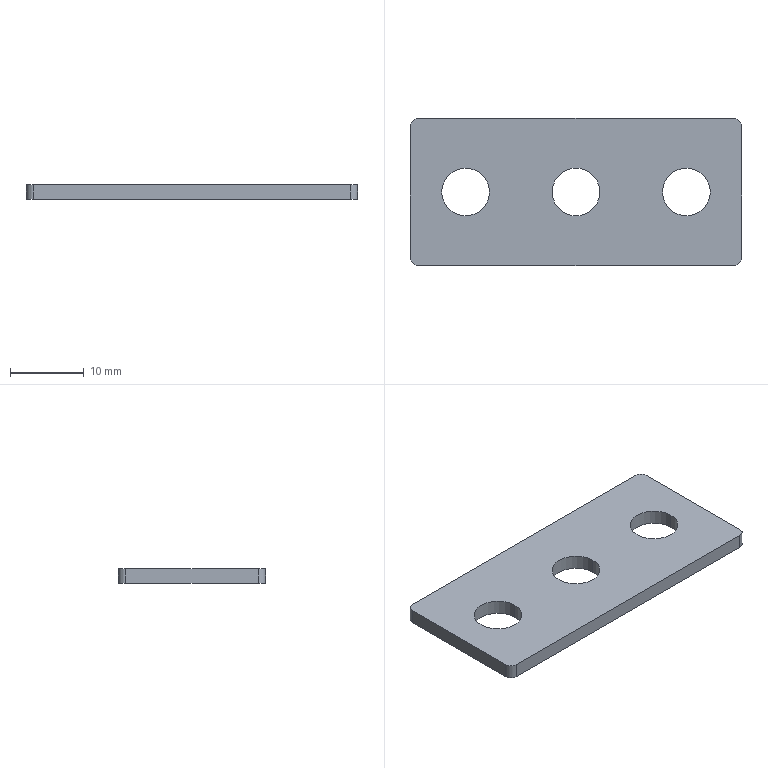Part | STEP file | 601-07-0010 | 1 solid | 16 faces | box 45 x 20 x 2 mm | volume 1599 mm3 | cylinder 10 | plane 6 | commonest cylinder face diameters 6.5 x6 2 x4
STEP:
#1=CARTESIAN_POINT('',(0.,0.,0.));
#2=DIRECTION('',(0.,0.,1.));
#3=DIRECTION('',(1.,0.,0.));
#4=AXIS2_PLACEMENT_3D('',#1,#2,#3);
#5=CARTESIAN_POINT('',(18.25,0.,0.));
#6=VERTEX_POINT('',#5);
#7=CARTESIAN_POINT('',(18.25,0.,2.));
#8=VERTEX_POINT('',#7);
#9=CARTESIAN_POINT('',(18.25,0.,0.));
#10=DIRECTION('',(0.,0.,1.));
#11=VECTOR('',#10,1.);
#12=LINE('',#9,#11);
#13=CARTESIAN_POINT('',(15.,0.,0.));
#14=DIRECTION('',(0.,0.,1.));
#15=DIRECTION('',(1.,0.,0.));
#16=AXIS2_PLACEMENT_3D('',#13,#14,#15);
#17=CYLINDRICAL_SURFACE('',#16,3.25);
#18=CARTESIAN_POINT('',(6.283,0.));
#19=DIRECTION('',(0.,1.));
#20=VECTOR('',#19,1.);
#21=LINE('',#18,#20);
#22=(GEOMETRIC_REPRESENTATION_CONTEXT(2)PARAMETRIC_REPRESENTATION_CONTEXT()REPRESENTATION_CONTEXT('',''));
#23=DEFINITIONAL_REPRESENTATION('',(#21),#22);
#24=PCURVE('',#17,#23);
#25=CARTESIAN_POINT('',(15.,0.,0.));
#26=DIRECTION('',(0.,0.,1.));
#27=DIRECTION('',(1.,0.,0.));
#28=AXIS2_PLACEMENT_3D('',#25,#26,#27);
#29=CYLINDRICAL_SURFACE('',#28,3.25);
#30=CARTESIAN_POINT('',(0.,0.));
#31=DIRECTION('',(0.,1.));
#32=VECTOR('',#31,1.);
#33=LINE('',#30,#32);
#34=(GEOMETRIC_REPRESENTATION_CONTEXT(2)PARAMETRIC_REPRESENTATION_CONTEXT()REPRESENTATION_CONTEXT('',''));
#35=DEFINITIONAL_REPRESENTATION('',(#33),#34);
#36=PCURVE('',#29,#35);
#37=SURFACE_CURVE('',#12,(#24,#36),.PCURVE_S1.);
#38=EDGE_CURVE('',#6,#8,#37,.T.);
#39=ORIENTED_EDGE('',*,*,#38,.T.);
#40=CARTESIAN_POINT('',(11.75,0.,2.));
#41=VERTEX_POINT('',#40);
#42=CARTESIAN_POINT('',(15.,0.,2.));
#43=DIRECTION('',(0.,0.,1.));
#44=DIRECTION('',(1.,0.,0.));
#45=AXIS2_PLACEMENT_3D('',#42,#43,#44);
#46=CIRCLE('',#45,3.25);
#47=CARTESIAN_POINT('',(0.,2.));
#48=DIRECTION('',(1.,0.));
#49=VECTOR('',#48,1.);
#50=LINE('',#47,#49);
#51=(GEOMETRIC_REPRESENTATION_CONTEXT(2)PARAMETRIC_REPRESENTATION_CONTEXT()REPRESENTATION_CONTEXT('',''));
#52=DEFINITIONAL_REPRESENTATION('',(#50),#51);
#53=PCURVE('',#17,#52);
#54=CARTESIAN_POINT('',(22.5,-10.,2.));
#55=DIRECTION('',(0.,0.,1.));
#56=DIRECTION('',(1.,0.,0.));
#57=AXIS2_PLACEMENT_3D('',#54,#55,#56);
#58=PLANE('',#57);
#59=CARTESIAN_POINT('',(-7.5,10.));
#60=DIRECTION('',(1.,0.));
#61=AXIS2_PLACEMENT_2D('',#59,#60);
#62=CIRCLE('',#61,3.25);
#63=(GEOMETRIC_REPRESENTATION_CONTEXT(2)PARAMETRIC_REPRESENTATION_CONTEXT()REPRESENTATION_CONTEXT('',''));
#64=DEFINITIONAL_REPRESENTATION('',(#62),#63);
#65=PCURVE('',#58,#64);
#66=SURFACE_CURVE('',#46,(#53,#65),.PCURVE_S1.);
#67=EDGE_CURVE('',#41,#8,#66,.T.);
#68=ORIENTED_EDGE('',*,*,#67,.F.);
#69=CARTESIAN_POINT('',(11.75,0.,0.));
#70=VERTEX_POINT('',#69);
#71=CARTESIAN_POINT('',(11.75,0.,0.));
#72=DIRECTION('',(0.,0.,1.));
#73=VECTOR('',#72,1.);
#74=LINE('',#71,#73);
#75=CARTESIAN_POINT('',(3.142,0.));
#76=DIRECTION('',(0.,1.));
#77=VECTOR('',#76,1.);
#78=LINE('',#75,#77);
#79=(GEOMETRIC_REPRESENTATION_CONTEXT(2)PARAMETRIC_REPRESENTATION_CONTEXT()REPRESENTATION_CONTEXT('',''));
#80=DEFINITIONAL_REPRESENTATION('',(#78),#79);
#81=PCURVE('',#17,#80);
#82=CARTESIAN_POINT('',(3.142,0.));
#83=DIRECTION('',(0.,1.));
#84=VECTOR('',#83,1.);
#85=LINE('',#82,#84);
#86=(GEOMETRIC_REPRESENTATION_CONTEXT(2)PARAMETRIC_REPRESENTATION_CONTEXT()REPRESENTATION_CONTEXT('',''));
#87=DEFINITIONAL_REPRESENTATION('',(#85),#86);
#88=PCURVE('',#29,#87);
#89=SURFACE_CURVE('',#74,(#81,#88),.PCURVE_S1.);
#90=EDGE_CURVE('',#70,#41,#89,.T.);
#91=ORIENTED_EDGE('',*,*,#90,.F.);
#92=CARTESIAN_POINT('',(15.,0.,0.));
#93=DIRECTION('',(0.,0.,1.));
#94=DIRECTION('',(1.,0.,0.));
#95=AXIS2_PLACEMENT_3D('',#92,#93,#94);
#96=CIRCLE('',#95,3.25);
#97=CARTESIAN_POINT('',(0.,0.));
#98=DIRECTION('',(1.,0.));
#99=VECTOR('',#98,1.);
#100=LINE('',#97,#99);
#101=(GEOMETRIC_REPRESENTATION_CONTEXT(2)PARAMETRIC_REPRESENTATION_CONTEXT()REPRESENTATION_CONTEXT('',''));
#102=DEFINITIONAL_REPRESENTATION('',(#100),#101);
#103=PCURVE('',#17,#102);
#104=CARTESIAN_POINT('',(22.5,-10.,0.));
#105=DIRECTION('',(0.,0.,1.));
#106=DIRECTION('',(1.,0.,0.));
#107=AXIS2_PLACEMENT_3D('',#104,#105,#106);
#108=PLANE('',#107);
#109=CARTESIAN_POINT('',(-7.5,10.));
#110=DIRECTION('',(1.,0.));
#111=AXIS2_PLACEMENT_2D('',#109,#110);
#112=CIRCLE('',#111,3.25);
#113=(GEOMETRIC_REPRESENTATION_CONTEXT(2)PARAMETRIC_REPRESENTATION_CONTEXT()REPRESENTATION_CONTEXT('',''));
#114=DEFINITIONAL_REPRESENTATION('',(#112),#113);
#115=PCURVE('',#108,#114);
#116=SURFACE_CURVE('',#96,(#103,#115),.PCURVE_S1.);
#117=EDGE_CURVE('',#70,#6,#116,.T.);
#118=ORIENTED_EDGE('',*,*,#117,.T.);
#119=EDGE_LOOP('',(#39,#68,#91,#118));
#120=FACE_BOUND('',#119,.F.);
#121=ADVANCED_FACE('',(#120),#17,.F.);
#122=CARTESIAN_POINT('',(3.25,0.,0.));
#123=VERTEX_POINT('',#122);
#124=CARTESIAN_POINT('',(3.25,0.,2.));
#125=VERTEX_POINT('',#124);
#126=CARTESIAN_POINT('',(3.25,0.,0.));
#127=DIRECTION('',(0.,0.,1.));
#128=VECTOR('',#127,1.);
#129=LINE('',#126,#128);
#130=CARTESIAN_POINT('',(0.,0.,0.));
#131=DIRECTION('',(0.,0.,1.));
#132=DIRECTION('',(1.,0.,0.));
#133=AXIS2_PLACEMENT_3D('',#130,#131,#132);
#134=CYLINDRICAL_SURFACE('',#133,3.25);
#135=CARTESIAN_POINT('',(6.283,0.));
#136=DIRECTION('',(0.,1.));
#137=VECTOR('',#136,1.);
#138=LINE('',#135,#137);
#139=(GEOMETRIC_REPRESENTATION_CONTEXT(2)PARAMETRIC_REPRESENTATION_CONTEXT()REPRESENTATION_CONTEXT('',''));
#140=DEFINITIONAL_REPRESENTATION('',(#138),#139);
#141=PCURVE('',#134,#140);
#142=CARTESIAN_POINT('',(0.,0.,0.));
#143=DIRECTION('',(0.,0.,1.));
#144=DIRECTION('',(1.,0.,0.));
#145=AXIS2_PLACEMENT_3D('',#142,#143,#144);
#146=CYLINDRICAL_SURFACE('',#145,3.25);
#147=CARTESIAN_POINT('',(0.,0.));
#148=DIRECTION('',(0.,1.));
#149=VECTOR('',#148,1.);
#150=LINE('',#147,#149);
#151=(GEOMETRIC_REPRESENTATION_CONTEXT(2)PARAMETRIC_REPRESENTATION_CONTEXT()REPRESENTATION_CONTEXT('',''));
#152=DEFINITIONAL_REPRESENTATION('',(#150),#151);
#153=PCURVE('',#146,#152);
#154=SURFACE_CURVE('',#129,(#141,#153),.PCURVE_S1.);
#155=EDGE_CURVE('',#123,#125,#154,.T.);
#156=ORIENTED_EDGE('',*,*,#155,.T.);
#157=CARTESIAN_POINT('',(-3.25,0.,2.));
#158=VERTEX_POINT('',#157);
#159=CARTESIAN_POINT('',(0.,0.,2.));
#160=DIRECTION('',(0.,0.,1.));
#161=DIRECTION('',(1.,0.,0.));
#162=AXIS2_PLACEMENT_3D('',#159,#160,#161);
#163=CIRCLE('',#162,3.25);
#164=CARTESIAN_POINT('',(0.,2.));
#165=DIRECTION('',(1.,0.));
#166=VECTOR('',#165,1.);
#167=LINE('',#164,#166);
#168=(GEOMETRIC_REPRESENTATION_CONTEXT(2)PARAMETRIC_REPRESENTATION_CONTEXT()REPRESENTATION_CONTEXT('',''));
#169=DEFINITIONAL_REPRESENTATION('',(#167),#168);
#170=PCURVE('',#134,#169);
#171=CARTESIAN_POINT('',(-22.5,10.));
#172=DIRECTION('',(1.,0.));
#173=AXIS2_PLACEMENT_2D('',#171,#172);
#174=CIRCLE('',#173,3.25);
#175=(GEOMETRIC_REPRESENTATION_CONTEXT(2)PARAMETRIC_REPRESENTATION_CONTEXT()REPRESENTATION_CONTEXT('',''));
#176=DEFINITIONAL_REPRESENTATION('',(#174),#175);
#177=PCURVE('',#58,#176);
#178=SURFACE_CURVE('',#163,(#170,#177),.PCURVE_S1.);
#179=EDGE_CURVE('',#158,#125,#178,.T.);
#180=ORIENTED_EDGE('',*,*,#179,.F.);
#181=CARTESIAN_POINT('',(-3.25,0.,0.));
#182=VERTEX_POINT('',#181);
#183=CARTESIAN_POINT('',(-3.25,0.,0.));
#184=DIRECTION('',(0.,0.,1.));
#185=VECTOR('',#184,1.);
#186=LINE('',#183,#185);
#187=CARTESIAN_POINT('',(3.142,0.));
#188=DIRECTION('',(0.,1.));
#189=VECTOR('',#188,1.);
#190=LINE('',#187,#189);
#191=(GEOMETRIC_REPRESENTATION_CONTEXT(2)PARAMETRIC_REPRESENTATION_CONTEXT()REPRESENTATION_CONTEXT('',''));
#192=DEFINITIONAL_REPRESENTATION('',(#190),#191);
#193=PCURVE('',#134,#192);
#194=CARTESIAN_POINT('',(3.142,0.));
#195=DIRECTION('',(0.,1.));
#196=VECTOR('',#195,1.);
#197=LINE('',#194,#196);
#198=(GEOMETRIC_REPRESENTATION_CONTEXT(2)PARAMETRIC_REPRESENTATION_CONTEXT()REPRESENTATION_CONTEXT('',''));
#199=DEFINITIONAL_REPRESENTATION('',(#197),#198);
#200=PCURVE('',#146,#199);
#201=SURFACE_CURVE('',#186,(#193,#200),.PCURVE_S1.);
#202=EDGE_CURVE('',#182,#158,#201,.T.);
#203=ORIENTED_EDGE('',*,*,#202,.F.);
#204=CARTESIAN_POINT('',(0.,0.,0.));
#205=DIRECTION('',(0.,0.,1.));
#206=DIRECTION('',(1.,0.,0.));
#207=AXIS2_PLACEMENT_3D('',#204,#205,#206);
#208=CIRCLE('',#207,3.25);
#209=CARTESIAN_POINT('',(0.,0.));
#210=DIRECTION('',(1.,0.));
#211=VECTOR('',#210,1.);
#212=LINE('',#209,#211);
#213=(GEOMETRIC_REPRESENTATION_CONTEXT(2)PARAMETRIC_REPRESENTATION_CONTEXT()REPRESENTATION_CONTEXT('',''));
#214=DEFINITIONAL_REPRESENTATION('',(#212),#213);
#215=PCURVE('',#134,#214);
#216=CARTESIAN_POINT('',(-22.5,10.));
#217=DIRECTION('',(1.,0.));
#218=AXIS2_PLACEMENT_2D('',#216,#217);
#219=CIRCLE('',#218,3.25);
#220=(GEOMETRIC_REPRESENTATION_CONTEXT(2)PARAMETRIC_REPRESENTATION_CONTEXT()REPRESENTATION_CONTEXT('',''));
#221=DEFINITIONAL_REPRESENTATION('',(#219),#220);
#222=PCURVE('',#108,#221);
#223=SURFACE_CURVE('',#208,(#215,#222),.PCURVE_S1.);
#224=EDGE_CURVE('',#182,#123,#223,.T.);
#225=ORIENTED_EDGE('',*,*,#224,.T.);
#226=EDGE_LOOP('',(#156,#180,#203,#225));
#227=FACE_BOUND('',#226,.F.);
#228=ADVANCED_FACE('',(#227),#134,.F.);
#229=CARTESIAN_POINT('',(-11.75,0.,0.));
#230=VERTEX_POINT('',#229);
#231=CARTESIAN_POINT('',(-11.75,0.,2.));
#232=VERTEX_POINT('',#231);
#233=CARTESIAN_POINT('',(-11.75,0.,0.));
#234=DIRECTION('',(0.,0.,1.));
#235=VECTOR('',#234,1.);
#236=LINE('',#233,#235);
#237=CARTESIAN_POINT('',(-15.,0.,0.));
#238=DIRECTION('',(0.,0.,1.));
#239=DIRECTION('',(1.,0.,0.));
#240=AXIS2_PLACEMENT_3D('',#237,#238,#239);
#241=CYLINDRICAL_SURFACE('',#240,3.25);
#242=CARTESIAN_POINT('',(6.283,0.));
#243=DIRECTION('',(0.,1.));
#244=VECTOR('',#243,1.);
#245=LINE('',#242,#244);
#246=(GEOMETRIC_REPRESENTATION_CONTEXT(2)PARAMETRIC_REPRESENTATION_CONTEXT()REPRESENTATION_CONTEXT('',''));
#247=DEFINITIONAL_REPRESENTATION('',(#245),#246);
#248=PCURVE('',#241,#247);
#249=CARTESIAN_POINT('',(-15.,0.,0.));
#250=DIRECTION('',(0.,0.,1.));
#251=DIRECTION('',(1.,0.,0.));
#252=AXIS2_PLACEMENT_3D('',#249,#250,#251);
#253=CYLINDRICAL_SURFACE('',#252,3.25);
#254=CARTESIAN_POINT('',(0.,0.));
#255=DIRECTION('',(0.,1.));
#256=VECTOR('',#255,1.);
#257=LINE('',#254,#256);
#258=(GEOMETRIC_REPRESENTATION_CONTEXT(2)PARAMETRIC_REPRESENTATION_CONTEXT()REPRESENTATION_CONTEXT('',''));
#259=DEFINITIONAL_REPRESENTATION('',(#257),#258);
#260=PCURVE('',#253,#259);
#261=SURFACE_CURVE('',#236,(#248,#260),.PCURVE_S1.);
#262=EDGE_CURVE('',#230,#232,#261,.T.);
#263=ORIENTED_EDGE('',*,*,#262,.T.);
#264=CARTESIAN_POINT('',(-18.25,0.,2.));
#265=VERTEX_POINT('',#264);
#266=CARTESIAN_POINT('',(-15.,0.,2.));
#267=DIRECTION('',(0.,0.,1.));
#268=DIRECTION('',(1.,0.,0.));
#269=AXIS2_PLACEMENT_3D('',#266,#267,#268);
#270=CIRCLE('',#269,3.25);
#271=CARTESIAN_POINT('',(0.,2.));
#272=DIRECTION('',(1.,0.));
#273=VECTOR('',#272,1.);
#274=LINE('',#271,#273);
#275=(GEOMETRIC_REPRESENTATION_CONTEXT(2)PARAMETRIC_REPRESENTATION_CONTEXT()REPRESENTATION_CONTEXT('',''));
#276=DEFINITIONAL_REPRESENTATION('',(#274),#275);
#277=PCURVE('',#241,#276);
#278=CARTESIAN_POINT('',(-37.5,10.));
#279=DIRECTION('',(1.,0.));
#280=AXIS2_PLACEMENT_2D('',#278,#279);
#281=CIRCLE('',#280,3.25);
#282=(GEOMETRIC_REPRESENTATION_CONTEXT(2)PARAMETRIC_REPRESENTATION_CONTEXT()REPRESENTATION_CONTEXT('',''));
#283=DEFINITIONAL_REPRESENTATION('',(#281),#282);
#284=PCURVE('',#58,#283);
#285=SURFACE_CURVE('',#270,(#277,#284),.PCURVE_S1.);
#286=EDGE_CURVE('',#265,#232,#285,.T.);
#287=ORIENTED_EDGE('',*,*,#286,.F.);
#288=CARTESIAN_POINT('',(-18.25,0.,0.));
#289=VERTEX_POINT('',#288);
#290=CARTESIAN_POINT('',(-18.25,0.,0.));
#291=DIRECTION('',(0.,0.,1.));
#292=VECTOR('',#291,1.);
#293=LINE('',#290,#292);
#294=CARTESIAN_POINT('',(3.142,0.));
#295=DIRECTION('',(0.,1.));
#296=VECTOR('',#295,1.);
#297=LINE('',#294,#296);
#298=(GEOMETRIC_REPRESENTATION_CONTEXT(2)PARAMETRIC_REPRESENTATION_CONTEXT()REPRESENTATION_CONTEXT('',''));
#299=DEFINITIONAL_REPRESENTATION('',(#297),#298);
#300=PCURVE('',#241,#299);
#301=CARTESIAN_POINT('',(3.142,0.));
#302=DIRECTION('',(0.,1.));
#303=VECTOR('',#302,1.);
#304=LINE('',#301,#303);
#305=(GEOMETRIC_REPRESENTATION_CONTEXT(2)PARAMETRIC_REPRESENTATION_CONTEXT()REPRESENTATION_CONTEXT('',''));
#306=DEFINITIONAL_REPRESENTATION('',(#304),#305);
#307=PCURVE('',#253,#306);
#308=SURFACE_CURVE('',#293,(#300,#307),.PCURVE_S1.);
#309=EDGE_CURVE('',#289,#265,#308,.T.);
#310=ORIENTED_EDGE('',*,*,#309,.F.);
#311=CARTESIAN_POINT('',(-15.,0.,0.));
#312=DIRECTION('',(0.,0.,1.));
#313=DIRECTION('',(1.,0.,0.));
#314=AXIS2_PLACEMENT_3D('',#311,#312,#313);
#315=CIRCLE('',#314,3.25);
#316=CARTESIAN_POINT('',(0.,0.));
#317=DIRECTION('',(1.,0.));
#318=VECTOR('',#317,1.);
#319=LINE('',#316,#318);
#320=(GEOMETRIC_REPRESENTATION_CONTEXT(2)PARAMETRIC_REPRESENTATION_CONTEXT()REPRESENTATION_CONTEXT('',''));
#321=DEFINITIONAL_REPRESENTATION('',(#319),#320);
#322=PCURVE('',#241,#321);
#323=CARTESIAN_POINT('',(-37.5,10.));
#324=DIRECTION('',(1.,0.));
#325=AXIS2_PLACEMENT_2D('',#323,#324);
#326=CIRCLE('',#325,3.25);
#327=(GEOMETRIC_REPRESENTATION_CONTEXT(2)PARAMETRIC_REPRESENTATION_CONTEXT()REPRESENTATION_CONTEXT('',''));
#328=DEFINITIONAL_REPRESENTATION('',(#326),#327);
#329=PCURVE('',#108,#328);
#330=SURFACE_CURVE('',#315,(#322,#329),.PCURVE_S1.);
#331=EDGE_CURVE('',#289,#230,#330,.T.);
#332=ORIENTED_EDGE('',*,*,#331,.T.);
#333=EDGE_LOOP('',(#263,#287,#310,#332));
#334=FACE_BOUND('',#333,.F.);
#335=ADVANCED_FACE('',(#334),#241,.F.);
#336=CARTESIAN_POINT('',(22.5,-9.,0.));
#337=VERTEX_POINT('',#336);
#338=CARTESIAN_POINT('',(22.5,9.,0.));
#339=VERTEX_POINT('',#338);
#340=CARTESIAN_POINT('',(22.5,10.,0.));
#341=DIRECTION('',(0.,1.,0.));
#342=VECTOR('',#341,1.);
#343=LINE('',#340,#342);
#344=CARTESIAN_POINT('',(22.5,10.,2.));
#345=DIRECTION('',(-1.,0.,0.));
#346=DIRECTION('',(0.,-1.,0.));
#347=AXIS2_PLACEMENT_3D('',#344,#345,#346);
#348=PLANE('',#347);
#349=CARTESIAN_POINT('',(0.,-2.));
#350=DIRECTION('',(-1.,0.));
#351=VECTOR('',#350,1.);
#352=LINE('',#349,#351);
#353=(GEOMETRIC_REPRESENTATION_CONTEXT(2)PARAMETRIC_REPRESENTATION_CONTEXT()REPRESENTATION_CONTEXT('',''));
#354=DEFINITIONAL_REPRESENTATION('',(#352),#353);
#355=PCURVE('',#348,#354);
#356=CARTESIAN_POINT('',(0.,20.));
#357=DIRECTION('',(0.,1.));
#358=VECTOR('',#357,1.);
#359=LINE('',#356,#358);
#360=(GEOMETRIC_REPRESENTATION_CONTEXT(2)PARAMETRIC_REPRESENTATION_CONTEXT()REPRESENTATION_CONTEXT('',''));
#361=DEFINITIONAL_REPRESENTATION('',(#359),#360);
#362=PCURVE('',#108,#361);
#363=SURFACE_CURVE('',#343,(#355,#362),.PCURVE_S1.);
#364=EDGE_CURVE('',#337,#339,#363,.T.);
#365=ORIENTED_EDGE('',*,*,#364,.T.);
#366=CARTESIAN_POINT('',(22.5,9.,2.));
#367=VERTEX_POINT('',#366);
#368=CARTESIAN_POINT('',(22.5,9.,2.));
#369=DIRECTION('',(0.,0.,1.));
#370=VECTOR('',#369,1.);
#371=LINE('',#368,#370);
#372=CARTESIAN_POINT('',(1.,0.));
#373=DIRECTION('',(0.,1.));
#374=VECTOR('',#373,1.);
#375=LINE('',#372,#374);
#376=(GEOMETRIC_REPRESENTATION_CONTEXT(2)PARAMETRIC_REPRESENTATION_CONTEXT()REPRESENTATION_CONTEXT('',''));
#377=DEFINITIONAL_REPRESENTATION('',(#375),#376);
#378=PCURVE('',#348,#377);
#379=CARTESIAN_POINT('',(21.5,9.,2.));
#380=DIRECTION('',(0.,0.,-1.));
#381=DIRECTION('',(-1.,0.,0.));
#382=AXIS2_PLACEMENT_3D('',#379,#380,#381);
#383=CYLINDRICAL_SURFACE('',#382,1.);
#384=CARTESIAN_POINT('',(3.142,0.));
#385=DIRECTION('',(0.,-1.));
#386=VECTOR('',#385,1.);
#387=LINE('',#384,#386);
#388=(GEOMETRIC_REPRESENTATION_CONTEXT(2)PARAMETRIC_REPRESENTATION_CONTEXT()REPRESENTATION_CONTEXT('',''));
#389=DEFINITIONAL_REPRESENTATION('',(#387),#388);
#390=PCURVE('',#383,#389);
#391=SURFACE_CURVE('',#371,(#378,#390),.PCURVE_S1.);
#392=EDGE_CURVE('',#339,#367,#391,.T.);
#393=ORIENTED_EDGE('',*,*,#392,.T.);
#394=CARTESIAN_POINT('',(22.5,-9.,2.));
#395=VERTEX_POINT('',#394);
#396=CARTESIAN_POINT('',(22.5,10.,2.));
#397=DIRECTION('',(0.,1.,0.));
#398=VECTOR('',#397,1.);
#399=LINE('',#396,#398);
#400=CARTESIAN_POINT('',(0.,0.));
#401=DIRECTION('',(-1.,0.));
#402=VECTOR('',#401,1.);
#403=LINE('',#400,#402);
#404=(GEOMETRIC_REPRESENTATION_CONTEXT(2)PARAMETRIC_REPRESENTATION_CONTEXT()REPRESENTATION_CONTEXT('',''));
#405=DEFINITIONAL_REPRESENTATION('',(#403),#404);
#406=PCURVE('',#348,#405);
#407=CARTESIAN_POINT('',(0.,20.));
#408=DIRECTION('',(0.,1.));
#409=VECTOR('',#408,1.);
#410=LINE('',#407,#409);
#411=(GEOMETRIC_REPRESENTATION_CONTEXT(2)PARAMETRIC_REPRESENTATION_CONTEXT()REPRESENTATION_CONTEXT('',''));
#412=DEFINITIONAL_REPRESENTATION('',(#410),#411);
#413=PCURVE('',#58,#412);
#414=SURFACE_CURVE('',#399,(#406,#413),.PCURVE_S1.);
#415=EDGE_CURVE('',#395,#367,#414,.T.);
#416=ORIENTED_EDGE('',*,*,#415,.F.);
#417=CARTESIAN_POINT('',(22.5,-9.,2.));
#418=DIRECTION('',(0.,0.,-1.));
#419=VECTOR('',#418,1.);
#420=LINE('',#417,#419);
#421=CARTESIAN_POINT('',(19.,0.));
#422=DIRECTION('',(0.,-1.));
#423=VECTOR('',#422,1.);
#424=LINE('',#421,#423);
#425=(GEOMETRIC_REPRESENTATION_CONTEXT(2)PARAMETRIC_REPRESENTATION_CONTEXT()REPRESENTATION_CONTEXT('',''));
#426=DEFINITIONAL_REPRESENTATION('',(#424),#425);
#427=PCURVE('',#348,#426);
#428=CARTESIAN_POINT('',(21.5,-9.,2.));
#429=DIRECTION('',(0.,0.,-1.));
#430=DIRECTION('',(-1.,0.,0.));
#431=AXIS2_PLACEMENT_3D('',#428,#429,#430);
#432=CYLINDRICAL_SURFACE('',#431,1.);
#433=CARTESIAN_POINT('',(3.142,0.));
#434=DIRECTION('',(0.,1.));
#435=VECTOR('',#434,1.);
#436=LINE('',#433,#435);
#437=(GEOMETRIC_REPRESENTATION_CONTEXT(2)PARAMETRIC_REPRESENTATION_CONTEXT()REPRESENTATION_CONTEXT('',''));
#438=DEFINITIONAL_REPRESENTATION('',(#436),#437);
#439=PCURVE('',#432,#438);
#440=SURFACE_CURVE('',#420,(#427,#439),.PCURVE_S1.);
#441=EDGE_CURVE('',#395,#337,#440,.T.);
#442=ORIENTED_EDGE('',*,*,#441,.T.);
#443=EDGE_LOOP('',(#365,#393,#416,#442));
#444=FACE_BOUND('',#443,.T.);
#445=ADVANCED_FACE('',(#444),#348,.F.);
#446=CARTESIAN_POINT('',(21.5,10.,0.));
#447=VERTEX_POINT('',#446);
#448=CARTESIAN_POINT('',(-21.5,10.,0.));
#449=VERTEX_POINT('',#448);
#450=CARTESIAN_POINT('',(-22.5,10.,0.));
#451=DIRECTION('',(-1.,0.,0.));
#452=VECTOR('',#451,1.);
#453=LINE('',#450,#452);
#454=CARTESIAN_POINT('',(-22.5,10.,2.));
#455=DIRECTION('',(0.,-1.,0.));
#456=DIRECTION('',(0.,0.,-1.));
#457=AXIS2_PLACEMENT_3D('',#454,#455,#456);
#458=PLANE('',#457);
#459=CARTESIAN_POINT('',(2.,0.));
#460=DIRECTION('',(0.,-1.));
#461=VECTOR('',#460,1.);
#462=LINE('',#459,#461);
#463=(GEOMETRIC_REPRESENTATION_CONTEXT(2)PARAMETRIC_REPRESENTATION_CONTEXT()REPRESENTATION_CONTEXT('',''));
#464=DEFINITIONAL_REPRESENTATION('',(#462),#463);
#465=PCURVE('',#458,#464);
#466=CARTESIAN_POINT('',(-45.,20.));
#467=DIRECTION('',(-1.,0.));
#468=VECTOR('',#467,1.);
#469=LINE('',#466,#468);
#470=(GEOMETRIC_REPRESENTATION_CONTEXT(2)PARAMETRIC_REPRESENTATION_CONTEXT()REPRESENTATION_CONTEXT('',''));
#471=DEFINITIONAL_REPRESENTATION('',(#469),#470);
#472=PCURVE('',#108,#471);
#473=SURFACE_CURVE('',#453,(#465,#472),.PCURVE_S1.);
#474=EDGE_CURVE('',#447,#449,#473,.T.);
#475=ORIENTED_EDGE('',*,*,#474,.T.);
#476=CARTESIAN_POINT('',(-21.5,10.,2.));
#477=VERTEX_POINT('',#476);
#478=CARTESIAN_POINT('',(-21.5,10.,2.));
#479=DIRECTION('',(0.,0.,1.));
#480=VECTOR('',#479,1.);
#481=LINE('',#478,#480);
#482=CARTESIAN_POINT('',(0.,1.));
#483=DIRECTION('',(-1.,0.));
#484=VECTOR('',#483,1.);
#485=LINE('',#482,#484);
#486=(GEOMETRIC_REPRESENTATION_CONTEXT(2)PARAMETRIC_REPRESENTATION_CONTEXT()REPRESENTATION_CONTEXT('',''));
#487=DEFINITIONAL_REPRESENTATION('',(#485),#486);
#488=PCURVE('',#458,#487);
#489=CARTESIAN_POINT('',(-21.5,9.,2.));
#490=DIRECTION('',(0.,0.,-1.));
#491=DIRECTION('',(-1.,0.,0.));
#492=AXIS2_PLACEMENT_3D('',#489,#490,#491);
#493=CYLINDRICAL_SURFACE('',#492,1.);
#494=CARTESIAN_POINT('',(1.571,0.));
#495=DIRECTION('',(0.,-1.));
#496=VECTOR('',#495,1.);
#497=LINE('',#494,#496);
#498=(GEOMETRIC_REPRESENTATION_CONTEXT(2)PARAMETRIC_REPRESENTATION_CONTEXT()REPRESENTATION_CONTEXT('',''));
#499=DEFINITIONAL_REPRESENTATION('',(#497),#498);
#500=PCURVE('',#493,#499);
#501=SURFACE_CURVE('',#481,(#488,#500),.PCURVE_S1.);
#502=EDGE_CURVE('',#449,#477,#501,.T.);
#503=ORIENTED_EDGE('',*,*,#502,.T.);
#504=CARTESIAN_POINT('',(21.5,10.,2.));
#505=VERTEX_POINT('',#504);
#506=CARTESIAN_POINT('',(-22.5,10.,2.));
#507=DIRECTION('',(-1.,0.,0.));
#508=VECTOR('',#507,1.);
#509=LINE('',#506,#508);
#510=CARTESIAN_POINT('',(0.,0.));
#511=DIRECTION('',(0.,-1.));
#512=VECTOR('',#511,1.);
#513=LINE('',#510,#512);
#514=(GEOMETRIC_REPRESENTATION_CONTEXT(2)PARAMETRIC_REPRESENTATION_CONTEXT()REPRESENTATION_CONTEXT('',''));
#515=DEFINITIONAL_REPRESENTATION('',(#513),#514);
#516=PCURVE('',#458,#515);
#517=CARTESIAN_POINT('',(-45.,20.));
#518=DIRECTION('',(-1.,0.));
#519=VECTOR('',#518,1.);
#520=LINE('',#517,#519);
#521=(GEOMETRIC_REPRESENTATION_CONTEXT(2)PARAMETRIC_REPRESENTATION_CONTEXT()REPRESENTATION_CONTEXT('',''));
#522=DEFINITIONAL_REPRESENTATION('',(#520),#521);
#523=PCURVE('',#58,#522);
#524=SURFACE_CURVE('',#509,(#516,#523),.PCURVE_S1.);
#525=EDGE_CURVE('',#505,#477,#524,.T.);
#526=ORIENTED_EDGE('',*,*,#525,.F.);
#527=CARTESIAN_POINT('',(21.5,10.,2.));
#528=DIRECTION('',(0.,0.,-1.));
#529=VECTOR('',#528,1.);
#530=LINE('',#527,#529);
#531=CARTESIAN_POINT('',(0.,44.));
#532=DIRECTION('',(1.,0.));
#533=VECTOR('',#532,1.);
#534=LINE('',#531,#533);
#535=(GEOMETRIC_REPRESENTATION_CONTEXT(2)PARAMETRIC_REPRESENTATION_CONTEXT()REPRESENTATION_CONTEXT('',''));
#536=DEFINITIONAL_REPRESENTATION('',(#534),#535);
#537=PCURVE('',#458,#536);
#538=CARTESIAN_POINT('',(1.571,0.));
#539=DIRECTION('',(0.,1.));
#540=VECTOR('',#539,1.);
#541=LINE('',#538,#540);
#542=(GEOMETRIC_REPRESENTATION_CONTEXT(2)PARAMETRIC_REPRESENTATION_CONTEXT()REPRESENTATION_CONTEXT('',''));
#543=DEFINITIONAL_REPRESENTATION('',(#541),#542);
#544=PCURVE('',#383,#543);
#545=SURFACE_CURVE('',#530,(#537,#544),.PCURVE_S1.);
#546=EDGE_CURVE('',#505,#447,#545,.T.);
#547=ORIENTED_EDGE('',*,*,#546,.T.);
#548=EDGE_LOOP('',(#475,#503,#526,#547));
#549=FACE_BOUND('',#548,.T.);
#550=ADVANCED_FACE('',(#549),#458,.F.);
#551=CARTESIAN_POINT('',(-22.5,9.,0.));
#552=VERTEX_POINT('',#551);
#553=CARTESIAN_POINT('',(-22.5,-9.,0.));
#554=VERTEX_POINT('',#553);
#555=CARTESIAN_POINT('',(-22.5,10.,0.));
#556=DIRECTION('',(0.,-1.,0.));
#557=VECTOR('',#556,1.);
#558=LINE('',#555,#557);
#559=CARTESIAN_POINT('',(-22.5,10.,2.));
#560=DIRECTION('',(1.,0.,0.));
#561=DIRECTION('',(0.,1.,0.));
#562=AXIS2_PLACEMENT_3D('',#559,#560,#561);
#563=PLANE('',#562);
#564=CARTESIAN_POINT('',(0.,-2.));
#565=DIRECTION('',(-1.,0.));
#566=VECTOR('',#565,1.);
#567=LINE('',#564,#566);
#568=(GEOMETRIC_REPRESENTATION_CONTEXT(2)PARAMETRIC_REPRESENTATION_CONTEXT()REPRESENTATION_CONTEXT('',''));
#569=DEFINITIONAL_REPRESENTATION('',(#567),#568);
#570=PCURVE('',#563,#569);
#571=CARTESIAN_POINT('',(-45.,20.));
#572=DIRECTION('',(0.,-1.));
#573=VECTOR('',#572,1.);
#574=LINE('',#571,#573);
#575=(GEOMETRIC_REPRESENTATION_CONTEXT(2)PARAMETRIC_REPRESENTATION_CONTEXT()REPRESENTATION_CONTEXT('',''));
#576=DEFINITIONAL_REPRESENTATION('',(#574),#575);
#577=PCURVE('',#108,#576);
#578=SURFACE_CURVE('',#558,(#570,#577),.PCURVE_S1.);
#579=EDGE_CURVE('',#552,#554,#578,.T.);
#580=ORIENTED_EDGE('',*,*,#579,.T.);
#581=CARTESIAN_POINT('',(-22.5,-9.,2.));
#582=VERTEX_POINT('',#581);
#583=CARTESIAN_POINT('',(-22.5,-9.,2.));
#584=DIRECTION('',(0.,0.,1.));
#585=VECTOR('',#584,1.);
#586=LINE('',#583,#585);
#587=CARTESIAN_POINT('',(-19.,0.));
#588=DIRECTION('',(0.,1.));
#589=VECTOR('',#588,1.);
#590=LINE('',#587,#589);
#591=(GEOMETRIC_REPRESENTATION_CONTEXT(2)PARAMETRIC_REPRESENTATION_CONTEXT()REPRESENTATION_CONTEXT('',''));
#592=DEFINITIONAL_REPRESENTATION('',(#590),#591);
#593=PCURVE('',#563,#592);
#594=CARTESIAN_POINT('',(-21.5,-9.,2.));
#595=DIRECTION('',(0.,0.,-1.));
#596=DIRECTION('',(-1.,0.,0.));
#597=AXIS2_PLACEMENT_3D('',#594,#595,#596);
#598=CYLINDRICAL_SURFACE('',#597,1.);
#599=CARTESIAN_POINT('',(6.283,0.));
#600=DIRECTION('',(0.,-1.));
#601=VECTOR('',#600,1.);
#602=LINE('',#599,#601);
#603=(GEOMETRIC_REPRESENTATION_CONTEXT(2)PARAMETRIC_REPRESENTATION_CONTEXT()REPRESENTATION_CONTEXT('',''));
#604=DEFINITIONAL_REPRESENTATION('',(#602),#603);
#605=PCURVE('',#598,#604);
#606=SURFACE_CURVE('',#586,(#593,#605),.PCURVE_S1.);
#607=EDGE_CURVE('',#554,#582,#606,.T.);
#608=ORIENTED_EDGE('',*,*,#607,.T.);
#609=CARTESIAN_POINT('',(-22.5,9.,2.));
#610=VERTEX_POINT('',#609);
#611=CARTESIAN_POINT('',(-22.5,10.,2.));
#612=DIRECTION('',(0.,-1.,0.));
#613=VECTOR('',#612,1.);
#614=LINE('',#611,#613);
#615=CARTESIAN_POINT('',(0.,0.));
#616=DIRECTION('',(-1.,0.));
#617=VECTOR('',#616,1.);
#618=LINE('',#615,#617);
#619=(GEOMETRIC_REPRESENTATION_CONTEXT(2)PARAMETRIC_REPRESENTATION_CONTEXT()REPRESENTATION_CONTEXT('',''));
#620=DEFINITIONAL_REPRESENTATION('',(#618),#619);
#621=PCURVE('',#563,#620);
#622=CARTESIAN_POINT('',(-45.,20.));
#623=DIRECTION('',(0.,-1.));
#624=VECTOR('',#623,1.);
#625=LINE('',#622,#624);
#626=(GEOMETRIC_REPRESENTATION_CONTEXT(2)PARAMETRIC_REPRESENTATION_CONTEXT()REPRESENTATION_CONTEXT('',''));
#627=DEFINITIONAL_REPRESENTATION('',(#625),#626);
#628=PCURVE('',#58,#627);
#629=SURFACE_CURVE('',#614,(#621,#628),.PCURVE_S1.);
#630=EDGE_CURVE('',#610,#582,#629,.T.);
#631=ORIENTED_EDGE('',*,*,#630,.F.);
#632=CARTESIAN_POINT('',(-22.5,9.,2.));
#633=DIRECTION('',(0.,0.,-1.));
#634=VECTOR('',#633,1.);
#635=LINE('',#632,#634);
#636=CARTESIAN_POINT('',(-1.,0.));
#637=DIRECTION('',(0.,-1.));
#638=VECTOR('',#637,1.);
#639=LINE('',#636,#638);
#640=(GEOMETRIC_REPRESENTATION_CONTEXT(2)PARAMETRIC_REPRESENTATION_CONTEXT()REPRESENTATION_CONTEXT('',''));
#641=DEFINITIONAL_REPRESENTATION('',(#639),#640);
#642=PCURVE('',#563,#641);
#643=CARTESIAN_POINT('',(0.,0.));
#644=DIRECTION('',(0.,1.));
#645=VECTOR('',#644,1.);
#646=LINE('',#643,#645);
#647=(GEOMETRIC_REPRESENTATION_CONTEXT(2)PARAMETRIC_REPRESENTATION_CONTEXT()REPRESENTATION_CONTEXT('',''));
#648=DEFINITIONAL_REPRESENTATION('',(#646),#647);
#649=PCURVE('',#493,#648);
#650=SURFACE_CURVE('',#635,(#642,#649),.PCURVE_S1.);
#651=EDGE_CURVE('',#610,#552,#650,.T.);
#652=ORIENTED_EDGE('',*,*,#651,.T.);
#653=EDGE_LOOP('',(#580,#608,#631,#652));
#654=FACE_BOUND('',#653,.T.);
#655=ADVANCED_FACE('',(#654),#563,.F.);
#656=CARTESIAN_POINT('',(-21.5,-10.,2.));
#657=VERTEX_POINT('',#656);
#658=CARTESIAN_POINT('',(21.5,-10.,2.));
#659=VERTEX_POINT('',#658);
#660=CARTESIAN_POINT('',(-22.5,-10.,2.));
#661=DIRECTION('',(1.,0.,0.));
#662=VECTOR('',#661,1.);
#663=LINE('',#660,#662);
#664=CARTESIAN_POINT('',(-22.5,-10.,2.));
#665=DIRECTION('',(0.,1.,0.));
#666=DIRECTION('',(0.,0.,1.));
#667=AXIS2_PLACEMENT_3D('',#664,#665,#666);
#668=PLANE('',#667);
#669=CARTESIAN_POINT('',(0.,0.));
#670=DIRECTION('',(0.,1.));
#671=VECTOR('',#670,1.);
#672=LINE('',#669,#671);
#673=(GEOMETRIC_REPRESENTATION_CONTEXT(2)PARAMETRIC_REPRESENTATION_CONTEXT()REPRESENTATION_CONTEXT('',''));
#674=DEFINITIONAL_REPRESENTATION('',(#672),#673);
#675=PCURVE('',#668,#674);
#676=CARTESIAN_POINT('',(-45.,0.));
#677=DIRECTION('',(1.,0.));
#678=VECTOR('',#677,1.);
#679=LINE('',#676,#678);
#680=(GEOMETRIC_REPRESENTATION_CONTEXT(2)PARAMETRIC_REPRESENTATION_CONTEXT()REPRESENTATION_CONTEXT('',''));
#681=DEFINITIONAL_REPRESENTATION('',(#679),#680);
#682=PCURVE('',#58,#681);
#683=SURFACE_CURVE('',#663,(#675,#682),.PCURVE_S1.);
#684=EDGE_CURVE('',#657,#659,#683,.T.);
#685=ORIENTED_EDGE('',*,*,#684,.F.);
#686=CARTESIAN_POINT('',(-21.5,-10.,0.));
#687=VERTEX_POINT('',#686);
#688=CARTESIAN_POINT('',(-21.5,-10.,2.));
#689=DIRECTION('',(0.,0.,-1.));
#690=VECTOR('',#689,1.);
#691=LINE('',#688,#690);
#692=CARTESIAN_POINT('',(0.,1.));
#693=DIRECTION('',(-1.,0.));
#694=VECTOR('',#693,1.);
#695=LINE('',#692,#694);
#696=(GEOMETRIC_REPRESENTATION_CONTEXT(2)PARAMETRIC_REPRESENTATION_CONTEXT()REPRESENTATION_CONTEXT('',''));
#697=DEFINITIONAL_REPRESENTATION('',(#695),#696);
#698=PCURVE('',#668,#697);
#699=CARTESIAN_POINT('',(4.712,0.));
#700=DIRECTION('',(0.,1.));
#701=VECTOR('',#700,1.);
#702=LINE('',#699,#701);
#703=(GEOMETRIC_REPRESENTATION_CONTEXT(2)PARAMETRIC_REPRESENTATION_CONTEXT()REPRESENTATION_CONTEXT('',''));
#704=DEFINITIONAL_REPRESENTATION('',(#702),#703);
#705=PCURVE('',#598,#704);
#706=SURFACE_CURVE('',#691,(#698,#705),.PCURVE_S1.);
#707=EDGE_CURVE('',#657,#687,#706,.T.);
#708=ORIENTED_EDGE('',*,*,#707,.T.);
#709=CARTESIAN_POINT('',(21.5,-10.,0.));
#710=VERTEX_POINT('',#709);
#711=CARTESIAN_POINT('',(-22.5,-10.,0.));
#712=DIRECTION('',(1.,0.,0.));
#713=VECTOR('',#712,1.);
#714=LINE('',#711,#713);
#715=CARTESIAN_POINT('',(-2.,0.));
#716=DIRECTION('',(0.,1.));
#717=VECTOR('',#716,1.);
#718=LINE('',#715,#717);
#719=(GEOMETRIC_REPRESENTATION_CONTEXT(2)PARAMETRIC_REPRESENTATION_CONTEXT()REPRESENTATION_CONTEXT('',''));
#720=DEFINITIONAL_REPRESENTATION('',(#718),#719);
#721=PCURVE('',#668,#720);
#722=CARTESIAN_POINT('',(-45.,0.));
#723=DIRECTION('',(1.,0.));
#724=VECTOR('',#723,1.);
#725=LINE('',#722,#724);
#726=(GEOMETRIC_REPRESENTATION_CONTEXT(2)PARAMETRIC_REPRESENTATION_CONTEXT()REPRESENTATION_CONTEXT('',''));
#727=DEFINITIONAL_REPRESENTATION('',(#725),#726);
#728=PCURVE('',#108,#727);
#729=SURFACE_CURVE('',#714,(#721,#728),.PCURVE_S1.);
#730=EDGE_CURVE('',#687,#710,#729,.T.);
#731=ORIENTED_EDGE('',*,*,#730,.T.);
#732=CARTESIAN_POINT('',(21.5,-10.,2.));
#733=DIRECTION('',(0.,0.,1.));
#734=VECTOR('',#733,1.);
#735=LINE('',#732,#734);
#736=CARTESIAN_POINT('',(0.,44.));
#737=DIRECTION('',(1.,0.));
#738=VECTOR('',#737,1.);
#739=LINE('',#736,#738);
#740=(GEOMETRIC_REPRESENTATION_CONTEXT(2)PARAMETRIC_REPRESENTATION_CONTEXT()REPRESENTATION_CONTEXT('',''));
#741=DEFINITIONAL_REPRESENTATION('',(#739),#740);
#742=PCURVE('',#668,#741);
#743=CARTESIAN_POINT('',(4.712,0.));
#744=DIRECTION('',(0.,-1.));
#745=VECTOR('',#744,1.);
#746=LINE('',#743,#745);
#747=(GEOMETRIC_REPRESENTATION_CONTEXT(2)PARAMETRIC_REPRESENTATION_CONTEXT()REPRESENTATION_CONTEXT('',''));
#748=DEFINITIONAL_REPRESENTATION('',(#746),#747);
#749=PCURVE('',#432,#748);
#750=SURFACE_CURVE('',#735,(#742,#749),.PCURVE_S1.);
#751=EDGE_CURVE('',#710,#659,#750,.T.);
#752=ORIENTED_EDGE('',*,*,#751,.T.);
#753=EDGE_LOOP('',(#685,#708,#731,#752));
#754=FACE_BOUND('',#753,.T.);
#755=ADVANCED_FACE('',(#754),#668,.F.);
#756=CARTESIAN_POINT('',(15.,0.,2.));
#757=DIRECTION('',(0.,0.,1.));
#758=DIRECTION('',(1.,0.,0.));
#759=AXIS2_PLACEMENT_3D('',#756,#757,#758);
#760=CIRCLE('',#759,3.25);
#761=CARTESIAN_POINT('',(-7.5,10.));
#762=DIRECTION('',(1.,0.));
#763=AXIS2_PLACEMENT_2D('',#761,#762);
#764=CIRCLE('',#763,3.25);
#765=(GEOMETRIC_REPRESENTATION_CONTEXT(2)PARAMETRIC_REPRESENTATION_CONTEXT()REPRESENTATION_CONTEXT('',''));
#766=DEFINITIONAL_REPRESENTATION('',(#764),#765);
#767=PCURVE('',#58,#766);
#768=CARTESIAN_POINT('',(0.,2.));
#769=DIRECTION('',(1.,0.));
#770=VECTOR('',#769,1.);
#771=LINE('',#768,#770);
#772=(GEOMETRIC_REPRESENTATION_CONTEXT(2)PARAMETRIC_REPRESENTATION_CONTEXT()REPRESENTATION_CONTEXT('',''));
#773=DEFINITIONAL_REPRESENTATION('',(#771),#772);
#774=PCURVE('',#29,#773);
#775=SURFACE_CURVE('',#760,(#767,#774),.PCURVE_S1.);
#776=EDGE_CURVE('',#8,#41,#775,.T.);
#777=ORIENTED_EDGE('',*,*,#776,.F.);
#778=ORIENTED_EDGE('',*,*,#67,.F.);
#779=EDGE_LOOP('',(#777,#778));
#780=FACE_BOUND('',#779,.T.);
#781=CARTESIAN_POINT('',(0.,0.,2.));
#782=DIRECTION('',(0.,0.,1.));
#783=DIRECTION('',(1.,0.,0.));
#784=AXIS2_PLACEMENT_3D('',#781,#782,#783);
#785=CIRCLE('',#784,3.25);
#786=CARTESIAN_POINT('',(-22.5,10.));
#787=DIRECTION('',(1.,0.));
#788=AXIS2_PLACEMENT_2D('',#786,#787);
#789=CIRCLE('',#788,3.25);
#790=(GEOMETRIC_REPRESENTATION_CONTEXT(2)PARAMETRIC_REPRESENTATION_CONTEXT()REPRESENTATION_CONTEXT('',''));
#791=DEFINITIONAL_REPRESENTATION('',(#789),#790);
#792=PCURVE('',#58,#791);
#793=CARTESIAN_POINT('',(0.,2.));
#794=DIRECTION('',(1.,0.));
#795=VECTOR('',#794,1.);
#796=LINE('',#793,#795);
#797=(GEOMETRIC_REPRESENTATION_CONTEXT(2)PARAMETRIC_REPRESENTATION_CONTEXT()REPRESENTATION_CONTEXT('',''));
#798=DEFINITIONAL_REPRESENTATION('',(#796),#797);
#799=PCURVE('',#146,#798);
#800=SURFACE_CURVE('',#785,(#792,#799),.PCURVE_S1.);
#801=EDGE_CURVE('',#125,#158,#800,.T.);
#802=ORIENTED_EDGE('',*,*,#801,.F.);
#803=ORIENTED_EDGE('',*,*,#179,.F.);
#804=EDGE_LOOP('',(#802,#803));
#805=FACE_BOUND('',#804,.T.);
#806=CARTESIAN_POINT('',(-15.,0.,2.));
#807=DIRECTION('',(0.,0.,1.));
#808=DIRECTION('',(1.,0.,0.));
#809=AXIS2_PLACEMENT_3D('',#806,#807,#808);
#810=CIRCLE('',#809,3.25);
#811=CARTESIAN_POINT('',(-37.5,10.));
#812=DIRECTION('',(1.,0.));
#813=AXIS2_PLACEMENT_2D('',#811,#812);
#814=CIRCLE('',#813,3.25);
#815=(GEOMETRIC_REPRESENTATION_CONTEXT(2)PARAMETRIC_REPRESENTATION_CONTEXT()REPRESENTATION_CONTEXT('',''));
#816=DEFINITIONAL_REPRESENTATION('',(#814),#815);
#817=PCURVE('',#58,#816);
#818=CARTESIAN_POINT('',(0.,2.));
#819=DIRECTION('',(1.,0.));
#820=VECTOR('',#819,1.);
#821=LINE('',#818,#820);
#822=(GEOMETRIC_REPRESENTATION_CONTEXT(2)PARAMETRIC_REPRESENTATION_CONTEXT()REPRESENTATION_CONTEXT('',''));
#823=DEFINITIONAL_REPRESENTATION('',(#821),#822);
#824=PCURVE('',#253,#823);
#825=SURFACE_CURVE('',#810,(#817,#824),.PCURVE_S1.);
#826=EDGE_CURVE('',#232,#265,#825,.T.);
#827=ORIENTED_EDGE('',*,*,#826,.F.);
#828=ORIENTED_EDGE('',*,*,#286,.F.);
#829=EDGE_LOOP('',(#827,#828));
#830=FACE_BOUND('',#829,.T.);
#831=ORIENTED_EDGE('',*,*,#630,.T.);
#832=CARTESIAN_POINT('',(-21.5,-9.,2.));
#833=DIRECTION('',(0.,0.,1.));
#834=DIRECTION('',(1.,0.,0.));
#835=AXIS2_PLACEMENT_3D('',#832,#833,#834);
#836=CIRCLE('',#835,1.);
#837=CARTESIAN_POINT('',(-44.,1.));
#838=DIRECTION('',(1.,0.));
#839=AXIS2_PLACEMENT_2D('',#837,#838);
#840=CIRCLE('',#839,1.);
#841=(GEOMETRIC_REPRESENTATION_CONTEXT(2)PARAMETRIC_REPRESENTATION_CONTEXT()REPRESENTATION_CONTEXT('',''));
#842=DEFINITIONAL_REPRESENTATION('',(#840),#841);
#843=PCURVE('',#58,#842);
#844=CARTESIAN_POINT('',(9.425,0.));
#845=DIRECTION('',(-1.,0.));
#846=VECTOR('',#845,1.);
#847=LINE('',#844,#846);
#848=(GEOMETRIC_REPRESENTATION_CONTEXT(2)PARAMETRIC_REPRESENTATION_CONTEXT()REPRESENTATION_CONTEXT('',''));
#849=DEFINITIONAL_REPRESENTATION('',(#847),#848);
#850=PCURVE('',#598,#849);
#851=SURFACE_CURVE('',#836,(#843,#850),.PCURVE_S1.);
#852=EDGE_CURVE('',#582,#657,#851,.T.);
#853=ORIENTED_EDGE('',*,*,#852,.T.);
#854=ORIENTED_EDGE('',*,*,#684,.T.);
#855=CARTESIAN_POINT('',(21.5,-9.,2.));
#856=DIRECTION('',(0.,0.,1.));
#857=DIRECTION('',(1.,0.,0.));
#858=AXIS2_PLACEMENT_3D('',#855,#856,#857);
#859=CIRCLE('',#858,1.);
#860=CARTESIAN_POINT('',(-1.,1.));
#861=DIRECTION('',(1.,0.));
#862=AXIS2_PLACEMENT_2D('',#860,#861);
#863=CIRCLE('',#862,1.);
#864=(GEOMETRIC_REPRESENTATION_CONTEXT(2)PARAMETRIC_REPRESENTATION_CONTEXT()REPRESENTATION_CONTEXT('',''));
#865=DEFINITIONAL_REPRESENTATION('',(#863),#864);
#866=PCURVE('',#58,#865);
#867=CARTESIAN_POINT('',(9.425,0.));
#868=DIRECTION('',(-1.,0.));
#869=VECTOR('',#868,1.);
#870=LINE('',#867,#869);
#871=(GEOMETRIC_REPRESENTATION_CONTEXT(2)PARAMETRIC_REPRESENTATION_CONTEXT()REPRESENTATION_CONTEXT('',''));
#872=DEFINITIONAL_REPRESENTATION('',(#870),#871);
#873=PCURVE('',#432,#872);
#874=SURFACE_CURVE('',#859,(#866,#873),.PCURVE_S1.);
#875=EDGE_CURVE('',#659,#395,#874,.T.);
#876=ORIENTED_EDGE('',*,*,#875,.T.);
#877=ORIENTED_EDGE('',*,*,#415,.T.);
#878=CARTESIAN_POINT('',(21.5,9.,2.));
#879=DIRECTION('',(0.,0.,1.));
#880=DIRECTION('',(1.,0.,0.));
#881=AXIS2_PLACEMENT_3D('',#878,#879,#880);
#882=CIRCLE('',#881,1.);
#883=CARTESIAN_POINT('',(-1.,19.));
#884=DIRECTION('',(1.,0.));
#885=AXIS2_PLACEMENT_2D('',#883,#884);
#886=CIRCLE('',#885,1.);
#887=(GEOMETRIC_REPRESENTATION_CONTEXT(2)PARAMETRIC_REPRESENTATION_CONTEXT()REPRESENTATION_CONTEXT('',''));
#888=DEFINITIONAL_REPRESENTATION('',(#886),#887);
#889=PCURVE('',#58,#888);
#890=CARTESIAN_POINT('',(3.142,0.));
#891=DIRECTION('',(-1.,0.));
#892=VECTOR('',#891,1.);
#893=LINE('',#890,#892);
#894=(GEOMETRIC_REPRESENTATION_CONTEXT(2)PARAMETRIC_REPRESENTATION_CONTEXT()REPRESENTATION_CONTEXT('',''));
#895=DEFINITIONAL_REPRESENTATION('',(#893),#894);
#896=PCURVE('',#383,#895);
#897=SURFACE_CURVE('',#882,(#889,#896),.PCURVE_S1.);
#898=EDGE_CURVE('',#367,#505,#897,.T.);
#899=ORIENTED_EDGE('',*,*,#898,.T.);
#900=ORIENTED_EDGE('',*,*,#525,.T.);
#901=CARTESIAN_POINT('',(-21.5,9.,2.));
#902=DIRECTION('',(0.,0.,1.));
#903=DIRECTION('',(1.,0.,0.));
#904=AXIS2_PLACEMENT_3D('',#901,#902,#903);
#905=CIRCLE('',#904,1.);
#906=CARTESIAN_POINT('',(-44.,19.));
#907=DIRECTION('',(1.,0.));
#908=AXIS2_PLACEMENT_2D('',#906,#907);
#909=CIRCLE('',#908,1.);
#910=(GEOMETRIC_REPRESENTATION_CONTEXT(2)PARAMETRIC_REPRESENTATION_CONTEXT()REPRESENTATION_CONTEXT('',''));
#911=DEFINITIONAL_REPRESENTATION('',(#909),#910);
#912=PCURVE('',#58,#911);
#913=CARTESIAN_POINT('',(3.142,0.));
#914=DIRECTION('',(-1.,0.));
#915=VECTOR('',#914,1.);
#916=LINE('',#913,#915);
#917=(GEOMETRIC_REPRESENTATION_CONTEXT(2)PARAMETRIC_REPRESENTATION_CONTEXT()REPRESENTATION_CONTEXT('',''));
#918=DEFINITIONAL_REPRESENTATION('',(#916),#917);
#919=PCURVE('',#493,#918);
#920=SURFACE_CURVE('',#905,(#912,#919),.PCURVE_S1.);
#921=EDGE_CURVE('',#477,#610,#920,.T.);
#922=ORIENTED_EDGE('',*,*,#921,.T.);
#923=EDGE_LOOP('',(#831,#853,#854,#876,#877,#899,#900,#922));
#924=FACE_BOUND('',#923,.T.);
#925=ADVANCED_FACE('',(#780,#805,#830,#924),#58,.T.);
#926=CARTESIAN_POINT('',(15.,0.,0.));
#927=DIRECTION('',(0.,0.,1.));
#928=DIRECTION('',(1.,0.,0.));
#929=AXIS2_PLACEMENT_3D('',#926,#927,#928);
#930=CIRCLE('',#929,3.25);
#931=CARTESIAN_POINT('',(-7.5,10.));
#932=DIRECTION('',(1.,0.));
#933=AXIS2_PLACEMENT_2D('',#931,#932);
#934=CIRCLE('',#933,3.25);
#935=(GEOMETRIC_REPRESENTATION_CONTEXT(2)PARAMETRIC_REPRESENTATION_CONTEXT()REPRESENTATION_CONTEXT('',''));
#936=DEFINITIONAL_REPRESENTATION('',(#934),#935);
#937=PCURVE('',#108,#936);
#938=CARTESIAN_POINT('',(0.,0.));
#939=DIRECTION('',(1.,0.));
#940=VECTOR('',#939,1.);
#941=LINE('',#938,#940);
#942=(GEOMETRIC_REPRESENTATION_CONTEXT(2)PARAMETRIC_REPRESENTATION_CONTEXT()REPRESENTATION_CONTEXT('',''));
#943=DEFINITIONAL_REPRESENTATION('',(#941),#942);
#944=PCURVE('',#29,#943);
#945=SURFACE_CURVE('',#930,(#937,#944),.PCURVE_S1.);
#946=EDGE_CURVE('',#6,#70,#945,.T.);
#947=ORIENTED_EDGE('',*,*,#946,.T.);
#948=ORIENTED_EDGE('',*,*,#117,.T.);
#949=EDGE_LOOP('',(#947,#948));
#950=FACE_BOUND('',#949,.T.);
#951=CARTESIAN_POINT('',(0.,0.,0.));
#952=DIRECTION('',(0.,0.,1.));
#953=DIRECTION('',(1.,0.,0.));
#954=AXIS2_PLACEMENT_3D('',#951,#952,#953);
#955=CIRCLE('',#954,3.25);
#956=CARTESIAN_POINT('',(-22.5,10.));
#957=DIRECTION('',(1.,0.));
#958=AXIS2_PLACEMENT_2D('',#956,#957);
#959=CIRCLE('',#958,3.25);
#960=(GEOMETRIC_REPRESENTATION_CONTEXT(2)PARAMETRIC_REPRESENTATION_CONTEXT()REPRESENTATION_CONTEXT('',''));
#961=DEFINITIONAL_REPRESENTATION('',(#959),#960);
#962=PCURVE('',#108,#961);
#963=CARTESIAN_POINT('',(0.,0.));
#964=DIRECTION('',(1.,0.));
#965=VECTOR('',#964,1.);
#966=LINE('',#963,#965);
#967=(GEOMETRIC_REPRESENTATION_CONTEXT(2)PARAMETRIC_REPRESENTATION_CONTEXT()REPRESENTATION_CONTEXT('',''));
#968=DEFINITIONAL_REPRESENTATION('',(#966),#967);
#969=PCURVE('',#146,#968);
#970=SURFACE_CURVE('',#955,(#962,#969),.PCURVE_S1.);
#971=EDGE_CURVE('',#123,#182,#970,.T.);
#972=ORIENTED_EDGE('',*,*,#971,.T.);
#973=ORIENTED_EDGE('',*,*,#224,.T.);
#974=EDGE_LOOP('',(#972,#973));
#975=FACE_BOUND('',#974,.T.);
#976=CARTESIAN_POINT('',(-15.,0.,0.));
#977=DIRECTION('',(0.,0.,1.));
#978=DIRECTION('',(1.,0.,0.));
#979=AXIS2_PLACEMENT_3D('',#976,#977,#978);
#980=CIRCLE('',#979,3.25);
#981=CARTESIAN_POINT('',(-37.5,10.));
#982=DIRECTION('',(1.,0.));
#983=AXIS2_PLACEMENT_2D('',#981,#982);
#984=CIRCLE('',#983,3.25);
#985=(GEOMETRIC_REPRESENTATION_CONTEXT(2)PARAMETRIC_REPRESENTATION_CONTEXT()REPRESENTATION_CONTEXT('',''));
#986=DEFINITIONAL_REPRESENTATION('',(#984),#985);
#987=PCURVE('',#108,#986);
#988=CARTESIAN_POINT('',(0.,0.));
#989=DIRECTION('',(1.,0.));
#990=VECTOR('',#989,1.);
#991=LINE('',#988,#990);
#992=(GEOMETRIC_REPRESENTATION_CONTEXT(2)PARAMETRIC_REPRESENTATION_CONTEXT()REPRESENTATION_CONTEXT('',''));
#993=DEFINITIONAL_REPRESENTATION('',(#991),#992);
#994=PCURVE('',#253,#993);
#995=SURFACE_CURVE('',#980,(#987,#994),.PCURVE_S1.);
#996=EDGE_CURVE('',#230,#289,#995,.T.);
#997=ORIENTED_EDGE('',*,*,#996,.T.);
#998=ORIENTED_EDGE('',*,*,#331,.T.);
#999=EDGE_LOOP('',(#997,#998));
#1000=FACE_BOUND('',#999,.T.);
#1001=ORIENTED_EDGE('',*,*,#730,.F.);
#1002=CARTESIAN_POINT('',(-21.5,-9.,0.));
#1003=DIRECTION('',(0.,0.,-1.));
#1004=DIRECTION('',(1.,0.,0.));
#1005=AXIS2_PLACEMENT_3D('',#1002,#1003,#1004);
#1006=CIRCLE('',#1005,1.);
#1007=CARTESIAN_POINT('',(-43.,1.));
#1008=CARTESIAN_POINT('',(-43.,-0.7321));
#1009=CARTESIAN_POINT('',(-44.5,0.134));
#1010=CARTESIAN_POINT('',(-46.,1.));
#1011=CARTESIAN_POINT('',(-44.5,1.866));
#1012=CARTESIAN_POINT('',(-43.,2.732));
#1013=CARTESIAN_POINT('',(-43.,1.));
#1014=(BOUNDED_CURVE()B_SPLINE_CURVE(2,(#1007,#1008,#1009,#1010,#1011,#1012,#1013),.UNSPECIFIED.,.T.,.F.)B_SPLINE_CURVE_WITH_KNOTS((1,2,2,2,2,1),(-2.094,0.,2.094,4.189,6.283,8.378),.UNSPECIFIED.)CURVE()GEOMETRIC_REPRESENTATION_ITEM()RATIONAL_B_SPLINE_CURVE((1.,0.5,1.,0.5,1.,0.5,1.))REPRESENTATION_ITEM(''));
#1015=(GEOMETRIC_REPRESENTATION_CONTEXT(2)PARAMETRIC_REPRESENTATION_CONTEXT()REPRESENTATION_CONTEXT('',''));
#1016=DEFINITIONAL_REPRESENTATION('',(#1014),#1015);
#1017=PCURVE('',#108,#1016);
#1018=CARTESIAN_POINT('',(3.142,2.));
#1019=DIRECTION('',(1.,0.));
#1020=VECTOR('',#1019,1.);
#1021=LINE('',#1018,#1020);
#1022=(GEOMETRIC_REPRESENTATION_CONTEXT(2)PARAMETRIC_REPRESENTATION_CONTEXT()REPRESENTATION_CONTEXT('',''));
#1023=DEFINITIONAL_REPRESENTATION('',(#1021),#1022);
#1024=PCURVE('',#598,#1023);
#1025=SURFACE_CURVE('',#1006,(#1017,#1024),.PCURVE_S1.);
#1026=EDGE_CURVE('',#687,#554,#1025,.T.);
#1027=ORIENTED_EDGE('',*,*,#1026,.T.);
#1028=ORIENTED_EDGE('',*,*,#579,.F.);
#1029=CARTESIAN_POINT('',(-21.5,9.,0.));
#1030=DIRECTION('',(0.,0.,-1.));
#1031=DIRECTION('',(1.,0.,0.));
#1032=AXIS2_PLACEMENT_3D('',#1029,#1030,#1031);
#1033=CIRCLE('',#1032,1.);
#1034=CARTESIAN_POINT('',(-43.,19.));
#1035=CARTESIAN_POINT('',(-43.,17.268));
#1036=CARTESIAN_POINT('',(-44.5,18.134));
#1037=CARTESIAN_POINT('',(-46.,19.));
#1038=CARTESIAN_POINT('',(-44.5,19.866));
#1039=CARTESIAN_POINT('',(-43.,20.732));
#1040=CARTESIAN_POINT('',(-43.,19.));
#1041=(BOUNDED_CURVE()B_SPLINE_CURVE(2,(#1034,#1035,#1036,#1037,#1038,#1039,#1040),.UNSPECIFIED.,.T.,.F.)B_SPLINE_CURVE_WITH_KNOTS((1,2,2,2,2,1),(-2.094,0.,2.094,4.189,6.283,8.378),.UNSPECIFIED.)CURVE()GEOMETRIC_REPRESENTATION_ITEM()RATIONAL_B_SPLINE_CURVE((1.,0.5,1.,0.5,1.,0.5,1.))REPRESENTATION_ITEM(''));
#1042=(GEOMETRIC_REPRESENTATION_CONTEXT(2)PARAMETRIC_REPRESENTATION_CONTEXT()REPRESENTATION_CONTEXT('',''));
#1043=DEFINITIONAL_REPRESENTATION('',(#1041),#1042);
#1044=PCURVE('',#108,#1043);
#1045=CARTESIAN_POINT('',(-3.142,2.));
#1046=DIRECTION('',(1.,0.));
#1047=VECTOR('',#1046,1.);
#1048=LINE('',#1045,#1047);
#1049=(GEOMETRIC_REPRESENTATION_CONTEXT(2)PARAMETRIC_REPRESENTATION_CONTEXT()REPRESENTATION_CONTEXT('',''));
#1050=DEFINITIONAL_REPRESENTATION('',(#1048),#1049);
#1051=PCURVE('',#493,#1050);
#1052=SURFACE_CURVE('',#1033,(#1044,#1051),.PCURVE_S1.);
#1053=EDGE_CURVE('',#552,#449,#1052,.T.);
#1054=ORIENTED_EDGE('',*,*,#1053,.T.);
#1055=ORIENTED_EDGE('',*,*,#474,.F.);
#1056=CARTESIAN_POINT('',(21.5,9.,0.));
#1057=DIRECTION('',(0.,0.,-1.));
#1058=DIRECTION('',(1.,0.,0.));
#1059=AXIS2_PLACEMENT_3D('',#1056,#1057,#1058);
#1060=CIRCLE('',#1059,1.);
#1061=CARTESIAN_POINT('',(0.,19.));
#1062=CARTESIAN_POINT('',(0.,17.268));
#1063=CARTESIAN_POINT('',(-1.5,18.134));
#1064=CARTESIAN_POINT('',(-3.,19.));
#1065=CARTESIAN_POINT('',(-1.5,19.866));
#1066=CARTESIAN_POINT('',(0.,20.732));
#1067=CARTESIAN_POINT('',(0.,19.));
#1068=(BOUNDED_CURVE()B_SPLINE_CURVE(2,(#1061,#1062,#1063,#1064,#1065,#1066,#1067),.UNSPECIFIED.,.T.,.F.)B_SPLINE_CURVE_WITH_KNOTS((1,2,2,2,2,1),(-2.094,0.,2.094,4.189,6.283,8.378),.UNSPECIFIED.)CURVE()GEOMETRIC_REPRESENTATION_ITEM()RATIONAL_B_SPLINE_CURVE((1.,0.5,1.,0.5,1.,0.5,1.))REPRESENTATION_ITEM(''));
#1069=(GEOMETRIC_REPRESENTATION_CONTEXT(2)PARAMETRIC_REPRESENTATION_CONTEXT()REPRESENTATION_CONTEXT('',''));
#1070=DEFINITIONAL_REPRESENTATION('',(#1068),#1069);
#1071=PCURVE('',#108,#1070);
#1072=CARTESIAN_POINT('',(-3.142,2.));
#1073=DIRECTION('',(1.,0.));
#1074=VECTOR('',#1073,1.);
#1075=LINE('',#1072,#1074);
#1076=(GEOMETRIC_REPRESENTATION_CONTEXT(2)PARAMETRIC_REPRESENTATION_CONTEXT()REPRESENTATION_CONTEXT('',''));
#1077=DEFINITIONAL_REPRESENTATION('',(#1075),#1076);
#1078=PCURVE('',#383,#1077);
#1079=SURFACE_CURVE('',#1060,(#1071,#1078),.PCURVE_S1.);
#1080=EDGE_CURVE('',#447,#339,#1079,.T.);
#1081=ORIENTED_EDGE('',*,*,#1080,.T.);
#1082=ORIENTED_EDGE('',*,*,#364,.F.);
#1083=CARTESIAN_POINT('',(21.5,-9.,0.));
#1084=DIRECTION('',(0.,0.,-1.));
#1085=DIRECTION('',(1.,0.,0.));
#1086=AXIS2_PLACEMENT_3D('',#1083,#1084,#1085);
#1087=CIRCLE('',#1086,1.);
#1088=CARTESIAN_POINT('',(0.,1.));
#1089=CARTESIAN_POINT('',(0.,-0.7321));
#1090=CARTESIAN_POINT('',(-1.5,0.134));
#1091=CARTESIAN_POINT('',(-3.,1.));
#1092=CARTESIAN_POINT('',(-1.5,1.866));
#1093=CARTESIAN_POINT('',(0.,2.732));
#1094=CARTESIAN_POINT('',(0.,1.));
#1095=(BOUNDED_CURVE()B_SPLINE_CURVE(2,(#1088,#1089,#1090,#1091,#1092,#1093,#1094),.UNSPECIFIED.,.T.,.F.)B_SPLINE_CURVE_WITH_KNOTS((1,2,2,2,2,1),(-2.094,0.,2.094,4.189,6.283,8.378),.UNSPECIFIED.)CURVE()GEOMETRIC_REPRESENTATION_ITEM()RATIONAL_B_SPLINE_CURVE((1.,0.5,1.,0.5,1.,0.5,1.))REPRESENTATION_ITEM(''));
#1096=(GEOMETRIC_REPRESENTATION_CONTEXT(2)PARAMETRIC_REPRESENTATION_CONTEXT()REPRESENTATION_CONTEXT('',''));
#1097=DEFINITIONAL_REPRESENTATION('',(#1095),#1096);
#1098=PCURVE('',#108,#1097);
#1099=CARTESIAN_POINT('',(3.142,2.));
#1100=DIRECTION('',(1.,0.));
#1101=VECTOR('',#1100,1.);
#1102=LINE('',#1099,#1101);
#1103=(GEOMETRIC_REPRESENTATION_CONTEXT(2)PARAMETRIC_REPRESENTATION_CONTEXT()REPRESENTATION_CONTEXT('',''));
#1104=DEFINITIONAL_REPRESENTATION('',(#1102),#1103);
#1105=PCURVE('',#432,#1104);
#1106=SURFACE_CURVE('',#1087,(#1098,#1105),.PCURVE_S1.);
#1107=EDGE_CURVE('',#337,#710,#1106,.T.);
#1108=ORIENTED_EDGE('',*,*,#1107,.T.);
#1109=EDGE_LOOP('',(#1001,#1027,#1028,#1054,#1055,#1081,#1082,#1108));
#1110=FACE_BOUND('',#1109,.T.);
#1111=ADVANCED_FACE('',(#950,#975,#1000,#1110),#108,.F.);
#1112=ORIENTED_EDGE('',*,*,#826,.F.);
#1113=ORIENTED_EDGE('',*,*,#262,.F.);
#1114=ORIENTED_EDGE('',*,*,#996,.T.);
#1115=ORIENTED_EDGE('',*,*,#309,.T.);
#1116=EDGE_LOOP('',(#1112,#1113,#1114,#1115));
#1117=FACE_BOUND('',#1116,.F.);
#1118=ADVANCED_FACE('',(#1117),#253,.F.);
#1119=ORIENTED_EDGE('',*,*,#801,.F.);
#1120=ORIENTED_EDGE('',*,*,#155,.F.);
#1121=ORIENTED_EDGE('',*,*,#971,.T.);
#1122=ORIENTED_EDGE('',*,*,#202,.T.);
#1123=EDGE_LOOP('',(#1119,#1120,#1121,#1122));
#1124=FACE_BOUND('',#1123,.F.);
#1125=ADVANCED_FACE('',(#1124),#146,.F.);
#1126=ORIENTED_EDGE('',*,*,#776,.F.);
#1127=ORIENTED_EDGE('',*,*,#38,.F.);
#1128=ORIENTED_EDGE('',*,*,#946,.T.);
#1129=ORIENTED_EDGE('',*,*,#90,.T.);
#1130=EDGE_LOOP('',(#1126,#1127,#1128,#1129));
#1131=FACE_BOUND('',#1130,.F.);
#1132=ADVANCED_FACE('',(#1131),#29,.F.);
#1133=ORIENTED_EDGE('',*,*,#852,.F.);
#1134=ORIENTED_EDGE('',*,*,#607,.F.);
#1135=ORIENTED_EDGE('',*,*,#1026,.F.);
#1136=ORIENTED_EDGE('',*,*,#707,.F.);
#1137=EDGE_LOOP('',(#1133,#1134,#1135,#1136));
#1138=FACE_BOUND('',#1137,.T.);
#1139=ADVANCED_FACE('',(#1138),#598,.T.);
#1140=ORIENTED_EDGE('',*,*,#921,.F.);
#1141=ORIENTED_EDGE('',*,*,#502,.F.);
#1142=ORIENTED_EDGE('',*,*,#1053,.F.);
#1143=ORIENTED_EDGE('',*,*,#651,.F.);
#1144=EDGE_LOOP('',(#1140,#1141,#1142,#1143));
#1145=FACE_BOUND('',#1144,.T.);
#1146=ADVANCED_FACE('',(#1145),#493,.T.);
#1147=ORIENTED_EDGE('',*,*,#898,.F.);
#1148=ORIENTED_EDGE('',*,*,#392,.F.);
#1149=ORIENTED_EDGE('',*,*,#1080,.F.);
#1150=ORIENTED_EDGE('',*,*,#546,.F.);
#1151=EDGE_LOOP('',(#1147,#1148,#1149,#1150));
#1152=FACE_BOUND('',#1151,.T.);
#1153=ADVANCED_FACE('',(#1152),#383,.T.);
#1154=ORIENTED_EDGE('',*,*,#875,.F.);
#1155=ORIENTED_EDGE('',*,*,#751,.F.);
#1156=ORIENTED_EDGE('',*,*,#1107,.F.);
#1157=ORIENTED_EDGE('',*,*,#441,.F.);
#1158=EDGE_LOOP('',(#1154,#1155,#1156,#1157));
#1159=FACE_BOUND('',#1158,.T.);
#1160=ADVANCED_FACE('',(#1159),#432,.T.);
#1161=CLOSED_SHELL('',(#121,#228,#335,#445,#550,#655,#755,#925,#1111,#1118,#1125,#1132,#1139,#1146,#1153,#1160));
#1162=MANIFOLD_SOLID_BREP('',#1161);
#1163=(LENGTH_UNIT()NAMED_UNIT(*)SI_UNIT(.MILLI.,.METRE.));
#1164=UNCERTAINTY_MEASURE_WITH_UNIT(LENGTH_MEASURE(0.0000001),#1163,'','');
#1165=(NAMED_UNIT(*)PLANE_ANGLE_UNIT()SI_UNIT($,.RADIAN.));
#1166=(NAMED_UNIT(*)SI_UNIT($,.STERADIAN.)SOLID_ANGLE_UNIT());
#1167=(GEOMETRIC_REPRESENTATION_CONTEXT(3)GLOBAL_UNCERTAINTY_ASSIGNED_CONTEXT((#1164))GLOBAL_UNIT_ASSIGNED_CONTEXT((#1163,#1165,#1166))REPRESENTATION_CONTEXT('',''));
#1168=ADVANCED_BREP_SHAPE_REPRESENTATION('',(#4,#1162),#1167);